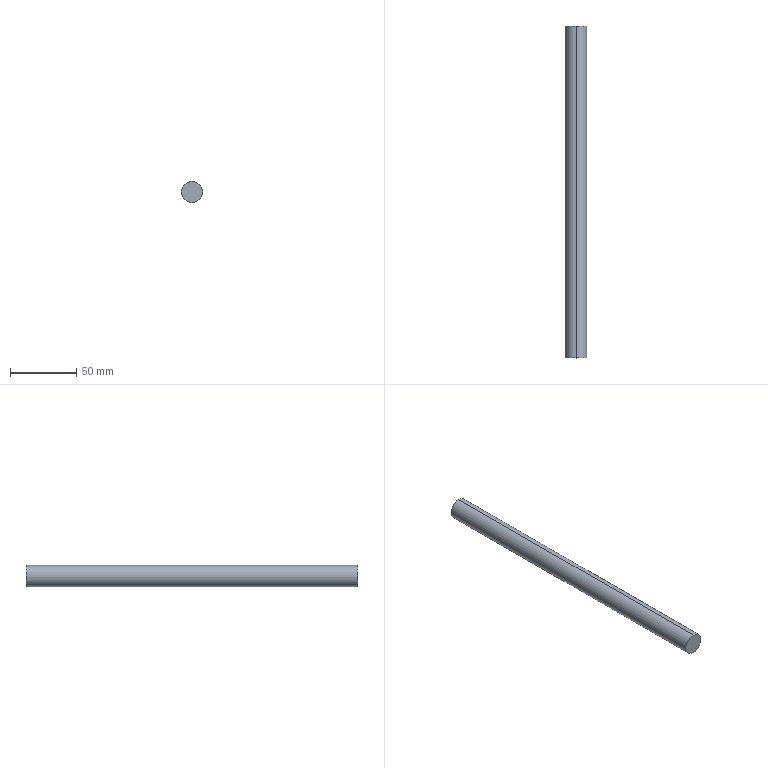Part | SolidWorks | features Extrusion 1, HoleWzd 1 | 1 solid | 8 faces | box 16 x 250 x 16 mm | volume 49961 mm3 | cylinder 4 | cone 2 | plane 2 | commonest cylinder face diameters 5 x2 16 x2
STEP:
#1=CARTESIAN_POINT('',(0.,235.,-2.5));
#2=VERTEX_POINT('',#1);
#3=CARTESIAN_POINT('',(0.,235.,2.5));
#4=VERTEX_POINT('',#3);
#5=CARTESIAN_POINT('',(0.,235.,0.));
#6=DIRECTION('',(0.,1.,0.));
#7=DIRECTION('',(0.,0.,1.));
#8=AXIS2_PLACEMENT_3D('',#5,#6,#7);
#9=CIRCLE('',#8,2.5);
#10=EDGE_CURVE('',#2,#4,#9,.T.);
#11=ORIENTED_EDGE('',*,*,#10,.F.);
#12=CARTESIAN_POINT('',(0.,250.,-2.5));
#13=VERTEX_POINT('',#12);
#14=CARTESIAN_POINT('',(0.,250.,-2.5));
#15=DIRECTION('',(0.,1.,0.));
#16=VECTOR('',#15,1000.);
#17=LINE('',#14,#16);
#18=EDGE_CURVE('',#2,#13,#17,.T.);
#19=ORIENTED_EDGE('',*,*,#18,.T.);
#20=CARTESIAN_POINT('',(0.,250.,2.5));
#21=VERTEX_POINT('',#20);
#22=CARTESIAN_POINT('',(0.,250.,0.));
#23=DIRECTION('',(0.,1.,0.));
#24=DIRECTION('',(0.,0.,1.));
#25=AXIS2_PLACEMENT_3D('',#22,#23,#24);
#26=CIRCLE('',#25,2.5);
#27=EDGE_CURVE('',#13,#21,#26,.T.);
#28=ORIENTED_EDGE('',*,*,#27,.T.);
#29=CARTESIAN_POINT('',(0.,250.,2.5));
#30=DIRECTION('',(0.,1.,0.));
#31=VECTOR('',#30,1000.);
#32=LINE('',#29,#31);
#33=EDGE_CURVE('',#4,#21,#32,.T.);
#34=ORIENTED_EDGE('',*,*,#33,.F.);
#35=EDGE_LOOP('',(#11,#19,#28,#34));
#36=FACE_OUTER_BOUND('',#35,.T.);
#37=CARTESIAN_POINT('',(0.,250.,0.));
#38=DIRECTION('',(0.,1.,0.));
#39=DIRECTION('',(0.,0.,1.));
#40=AXIS2_PLACEMENT_3D('',#37,#38,#39);
#41=CYLINDRICAL_SURFACE('',#40,2.5);
#42=ADVANCED_FACE('',(#36),#41,.F.);
#43=CARTESIAN_POINT('',(0.,233.498,0.));
#44=VERTEX_POINT('',#43);
#45=CARTESIAN_POINT('',(0.,235.,2.5));
#46=DIRECTION('',(0.,0.515,0.8572));
#47=VECTOR('',#46,1000.);
#48=LINE('',#45,#47);
#49=EDGE_CURVE('',#44,#4,#48,.T.);
#50=ORIENTED_EDGE('',*,*,#49,.F.);
#51=CARTESIAN_POINT('',(0.,235.,-2.5));
#52=DIRECTION('',(0.,0.515,-0.8572));
#53=VECTOR('',#52,1000.);
#54=LINE('',#51,#53);
#55=EDGE_CURVE('',#44,#2,#54,.T.);
#56=ORIENTED_EDGE('',*,*,#55,.T.);
#57=ORIENTED_EDGE('',*,*,#10,.T.);
#58=EDGE_LOOP('',(#50,#56,#57));
#59=FACE_OUTER_BOUND('',#58,.T.);
#60=CARTESIAN_POINT('',(0.,235.,0.));
#61=DIRECTION('',(0.,1.,0.));
#62=DIRECTION('',(0.,0.,1.));
#63=AXIS2_PLACEMENT_3D('',#60,#61,#62);
#64=CONICAL_SURFACE('',#63,2.5,1.03);
#65=ADVANCED_FACE('',(#59),#64,.F.);
#66=CARTESIAN_POINT('',(0.,250.,8.));
#67=VERTEX_POINT('',#66);
#68=CARTESIAN_POINT('',(0.,250.,-8.));
#69=VERTEX_POINT('',#68);
#70=CARTESIAN_POINT('',(0.,250.,0.));
#71=DIRECTION('',(0.,1.,0.));
#72=DIRECTION('',(0.,0.,1.));
#73=AXIS2_PLACEMENT_3D('',#70,#71,#72);
#74=CIRCLE('',#73,8.);
#75=EDGE_CURVE('',#67,#69,#74,.T.);
#76=ORIENTED_EDGE('',*,*,#75,.F.);
#77=CARTESIAN_POINT('',(0.,0.,8.));
#78=VERTEX_POINT('',#77);
#79=CARTESIAN_POINT('',(0.,250.,8.));
#80=DIRECTION('',(0.,-1.,0.));
#81=VECTOR('',#80,1000.);
#82=LINE('',#79,#81);
#83=EDGE_CURVE('',#67,#78,#82,.T.);
#84=ORIENTED_EDGE('',*,*,#83,.T.);
#85=CARTESIAN_POINT('',(0.,0.,-8.));
#86=VERTEX_POINT('',#85);
#87=CARTESIAN_POINT('',(0.,0.,0.));
#88=DIRECTION('',(0.,1.,0.));
#89=DIRECTION('',(0.,0.,1.));
#90=AXIS2_PLACEMENT_3D('',#87,#88,#89);
#91=CIRCLE('',#90,8.);
#92=EDGE_CURVE('',#78,#86,#91,.T.);
#93=ORIENTED_EDGE('',*,*,#92,.T.);
#94=CARTESIAN_POINT('',(0.,250.,-8.));
#95=DIRECTION('',(0.,-1.,0.));
#96=VECTOR('',#95,1000.);
#97=LINE('',#94,#96);
#98=EDGE_CURVE('',#69,#86,#97,.T.);
#99=ORIENTED_EDGE('',*,*,#98,.F.);
#100=EDGE_LOOP('',(#76,#84,#93,#99));
#101=FACE_OUTER_BOUND('',#100,.T.);
#102=CARTESIAN_POINT('',(0.,250.,0.));
#103=DIRECTION('',(0.,-1.,0.));
#104=DIRECTION('',(0.,0.,-1.));
#105=AXIS2_PLACEMENT_3D('',#102,#103,#104);
#106=CYLINDRICAL_SURFACE('',#105,8.);
#107=ADVANCED_FACE('',(#101),#106,.T.);
#108=ORIENTED_EDGE('',*,*,#83,.F.);
#109=CARTESIAN_POINT('',(0.,250.,0.));
#110=DIRECTION('',(0.,1.,0.));
#111=DIRECTION('',(0.,0.,1.));
#112=AXIS2_PLACEMENT_3D('',#109,#110,#111);
#113=CIRCLE('',#112,8.);
#114=EDGE_CURVE('',#69,#67,#113,.T.);
#115=ORIENTED_EDGE('',*,*,#114,.F.);
#116=ORIENTED_EDGE('',*,*,#98,.T.);
#117=CARTESIAN_POINT('',(0.,0.,0.));
#118=DIRECTION('',(0.,1.,0.));
#119=DIRECTION('',(0.,0.,1.));
#120=AXIS2_PLACEMENT_3D('',#117,#118,#119);
#121=CIRCLE('',#120,8.);
#122=EDGE_CURVE('',#86,#78,#121,.T.);
#123=ORIENTED_EDGE('',*,*,#122,.T.);
#124=EDGE_LOOP('',(#108,#115,#116,#123));
#125=FACE_OUTER_BOUND('',#124,.T.);
#126=CARTESIAN_POINT('',(0.,250.,0.));
#127=DIRECTION('',(0.,-1.,0.));
#128=DIRECTION('',(0.,0.,-1.));
#129=AXIS2_PLACEMENT_3D('',#126,#127,#128);
#130=CYLINDRICAL_SURFACE('',#129,8.);
#131=ADVANCED_FACE('',(#125),#130,.T.);
#132=CARTESIAN_POINT('',(0.,250.,0.));
#133=DIRECTION('',(0.,1.,0.));
#134=DIRECTION('',(0.,0.,1.));
#135=AXIS2_PLACEMENT_3D('',#132,#133,#134);
#136=CIRCLE('',#135,2.5);
#137=EDGE_CURVE('',#21,#13,#136,.T.);
#138=ORIENTED_EDGE('',*,*,#137,.F.);
#139=ORIENTED_EDGE('',*,*,#27,.F.);
#140=EDGE_LOOP('',(#138,#139));
#141=FACE_BOUND('',#140,.T.);
#142=ORIENTED_EDGE('',*,*,#114,.T.);
#143=ORIENTED_EDGE('',*,*,#75,.T.);
#144=EDGE_LOOP('',(#142,#143));
#145=FACE_OUTER_BOUND('',#144,.T.);
#146=CARTESIAN_POINT('',(0.,250.,0.));
#147=DIRECTION('',(0.,1.,0.));
#148=DIRECTION('',(0.,0.,1.));
#149=AXIS2_PLACEMENT_3D('',#146,#147,#148);
#150=PLANE('',#149);
#151=ADVANCED_FACE('',(#141,#145),#150,.T.);
#152=ORIENTED_EDGE('',*,*,#122,.F.);
#153=ORIENTED_EDGE('',*,*,#92,.F.);
#154=EDGE_LOOP('',(#152,#153));
#155=FACE_OUTER_BOUND('',#154,.T.);
#156=CARTESIAN_POINT('',(0.,0.,0.));
#157=DIRECTION('',(0.,1.,0.));
#158=DIRECTION('',(0.,0.,1.));
#159=AXIS2_PLACEMENT_3D('',#156,#157,#158);
#160=PLANE('',#159);
#161=ADVANCED_FACE('',(#155),#160,.F.);
#162=ORIENTED_EDGE('',*,*,#55,.F.);
#163=ORIENTED_EDGE('',*,*,#49,.T.);
#164=CARTESIAN_POINT('',(0.,235.,0.));
#165=DIRECTION('',(0.,1.,0.));
#166=DIRECTION('',(0.,0.,1.));
#167=AXIS2_PLACEMENT_3D('',#164,#165,#166);
#168=CIRCLE('',#167,2.5);
#169=EDGE_CURVE('',#4,#2,#168,.T.);
#170=ORIENTED_EDGE('',*,*,#169,.T.);
#171=EDGE_LOOP('',(#162,#163,#170));
#172=FACE_OUTER_BOUND('',#171,.T.);
#173=CARTESIAN_POINT('',(0.,235.,0.));
#174=DIRECTION('',(0.,1.,0.));
#175=DIRECTION('',(0.,0.,1.));
#176=AXIS2_PLACEMENT_3D('',#173,#174,#175);
#177=CONICAL_SURFACE('',#176,2.5,1.03);
#178=ADVANCED_FACE('',(#172),#177,.F.);
#179=ORIENTED_EDGE('',*,*,#18,.F.);
#180=ORIENTED_EDGE('',*,*,#169,.F.);
#181=ORIENTED_EDGE('',*,*,#33,.T.);
#182=ORIENTED_EDGE('',*,*,#137,.T.);
#183=EDGE_LOOP('',(#179,#180,#181,#182));
#184=FACE_OUTER_BOUND('',#183,.T.);
#185=CARTESIAN_POINT('',(0.,250.,0.));
#186=DIRECTION('',(0.,1.,0.));
#187=DIRECTION('',(0.,0.,1.));
#188=AXIS2_PLACEMENT_3D('',#185,#186,#187);
#189=CYLINDRICAL_SURFACE('',#188,2.5);
#190=ADVANCED_FACE('',(#184),#189,.F.);
#191=CLOSED_SHELL('',(#42,#65,#107,#131,#151,#161,#178,#190));
#192=MANIFOLD_SOLID_BREP('',#191);
#193=CARTESIAN_POINT('',(0.,0.,0.));
#194=DIRECTION('',(0.,0.,1.));
#195=DIRECTION('',(1.,0.,0.));
#196=AXIS2_PLACEMENT_3D('',#193,#194,#195);
#197=(LENGTH_UNIT()NAMED_UNIT(*)SI_UNIT(.MILLI.,.METRE.));
#198=UNCERTAINTY_MEASURE_WITH_UNIT(LENGTH_MEASURE(0.00001),#197,'','');
#199=(NAMED_UNIT(*)PLANE_ANGLE_UNIT()SI_UNIT($,.RADIAN.));
#200=(NAMED_UNIT(*)SI_UNIT($,.STERADIAN.)SOLID_ANGLE_UNIT());
#201=(GEOMETRIC_REPRESENTATION_CONTEXT(3)GLOBAL_UNCERTAINTY_ASSIGNED_CONTEXT((#198))GLOBAL_UNIT_ASSIGNED_CONTEXT((#197,#199,#200))REPRESENTATION_CONTEXT('',''));
#202=ADVANCED_BREP_SHAPE_REPRESENTATION('',(#192,#196),#201);